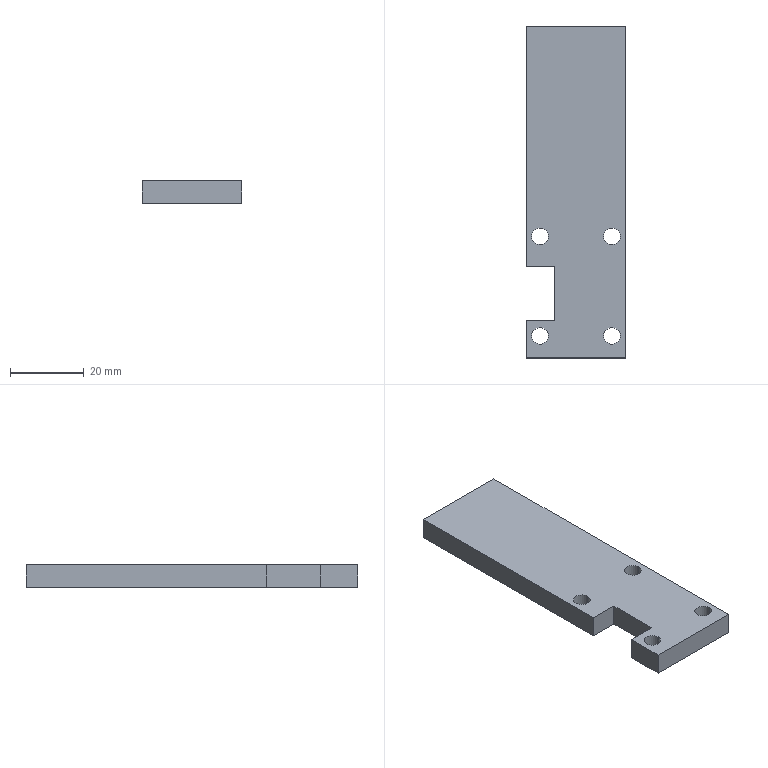Part | NX | features BREP 1 | 1 solid | 18 faces | box 27 x 90 x 6 mm | volume 13520 mm3 | plane 10 | cylinder 8 | commonest cylinder face diameters 4.5 x8
STEP:
#1=CARTESIAN_POINT('',(-758.389,33.,6.));
#2=VERTEX_POINT('',#1);
#3=CARTESIAN_POINT('',(-762.889,33.,6.));
#4=VERTEX_POINT('',#3);
#5=CARTESIAN_POINT('',(-760.639,33.,6.));
#6=DIRECTION('',(0.,0.,-1.));
#7=DIRECTION('',(-1.,0.,0.));
#8=AXIS2_PLACEMENT_3D('',#5,#6,#7);
#9=CIRCLE('',#8,2.25);
#10=EDGE_CURVE('',#2,#4,#9,.T.);
#11=ORIENTED_EDGE('',*,*,#10,.F.);
#12=CARTESIAN_POINT('',(-758.389,33.,0.));
#13=VERTEX_POINT('',#12);
#14=CARTESIAN_POINT('',(-758.389,33.,6.));
#15=DIRECTION('',(0.,0.,-1.));
#16=VECTOR('',#15,1000.);
#17=LINE('',#14,#16);
#18=EDGE_CURVE('',#2,#13,#17,.T.);
#19=ORIENTED_EDGE('',*,*,#18,.T.);
#20=CARTESIAN_POINT('',(-762.889,33.,0.));
#21=VERTEX_POINT('',#20);
#22=CARTESIAN_POINT('',(-760.639,33.,0.));
#23=DIRECTION('',(0.,0.,-1.));
#24=DIRECTION('',(-1.,0.,0.));
#25=AXIS2_PLACEMENT_3D('',#22,#23,#24);
#26=CIRCLE('',#25,2.25);
#27=EDGE_CURVE('',#13,#21,#26,.T.);
#28=ORIENTED_EDGE('',*,*,#27,.T.);
#29=CARTESIAN_POINT('',(-762.889,33.,6.));
#30=DIRECTION('',(0.,0.,-1.));
#31=VECTOR('',#30,1000.);
#32=LINE('',#29,#31);
#33=EDGE_CURVE('',#4,#21,#32,.T.);
#34=ORIENTED_EDGE('',*,*,#33,.F.);
#35=EDGE_LOOP('',(#11,#19,#28,#34));
#36=FACE_BOUND('',#35,.T.);
#37=CARTESIAN_POINT('',(-760.639,33.,6.));
#38=DIRECTION('',(0.,0.,-1.));
#39=DIRECTION('',(-1.,0.,0.));
#40=AXIS2_PLACEMENT_3D('',#37,#38,#39);
#41=CYLINDRICAL_SURFACE('',#40,2.25);
#42=ADVANCED_FACE('',(#36),#41,.F.);
#43=CARTESIAN_POINT('',(-758.389,6.,6.));
#44=VERTEX_POINT('',#43);
#45=CARTESIAN_POINT('',(-762.889,6.,6.));
#46=VERTEX_POINT('',#45);
#47=CARTESIAN_POINT('',(-760.639,6.,6.));
#48=DIRECTION('',(0.,0.,-1.));
#49=DIRECTION('',(-1.,0.,0.));
#50=AXIS2_PLACEMENT_3D('',#47,#48,#49);
#51=CIRCLE('',#50,2.25);
#52=EDGE_CURVE('',#44,#46,#51,.T.);
#53=ORIENTED_EDGE('',*,*,#52,.F.);
#54=CARTESIAN_POINT('',(-758.389,6.,0.));
#55=VERTEX_POINT('',#54);
#56=CARTESIAN_POINT('',(-758.389,6.,6.));
#57=DIRECTION('',(0.,0.,-1.));
#58=VECTOR('',#57,1000.);
#59=LINE('',#56,#58);
#60=EDGE_CURVE('',#44,#55,#59,.T.);
#61=ORIENTED_EDGE('',*,*,#60,.T.);
#62=CARTESIAN_POINT('',(-762.889,6.,0.));
#63=VERTEX_POINT('',#62);
#64=CARTESIAN_POINT('',(-760.639,6.,0.));
#65=DIRECTION('',(0.,0.,-1.));
#66=DIRECTION('',(-1.,0.,0.));
#67=AXIS2_PLACEMENT_3D('',#64,#65,#66);
#68=CIRCLE('',#67,2.25);
#69=EDGE_CURVE('',#55,#63,#68,.T.);
#70=ORIENTED_EDGE('',*,*,#69,.T.);
#71=CARTESIAN_POINT('',(-762.889,6.,6.));
#72=DIRECTION('',(0.,0.,-1.));
#73=VECTOR('',#72,1000.);
#74=LINE('',#71,#73);
#75=EDGE_CURVE('',#46,#63,#74,.T.);
#76=ORIENTED_EDGE('',*,*,#75,.F.);
#77=EDGE_LOOP('',(#53,#61,#70,#76));
#78=FACE_BOUND('',#77,.T.);
#79=CARTESIAN_POINT('',(-760.639,6.,6.));
#80=DIRECTION('',(0.,0.,-1.));
#81=DIRECTION('',(-1.,0.,0.));
#82=AXIS2_PLACEMENT_3D('',#79,#80,#81);
#83=CYLINDRICAL_SURFACE('',#82,2.25);
#84=ADVANCED_FACE('',(#78),#83,.F.);
#85=CARTESIAN_POINT('',(-777.889,6.,6.));
#86=VERTEX_POINT('',#85);
#87=CARTESIAN_POINT('',(-782.389,6.,6.));
#88=VERTEX_POINT('',#87);
#89=CARTESIAN_POINT('',(-780.139,6.,6.));
#90=DIRECTION('',(0.,0.,-1.));
#91=DIRECTION('',(-1.,0.,0.));
#92=AXIS2_PLACEMENT_3D('',#89,#90,#91);
#93=CIRCLE('',#92,2.25);
#94=EDGE_CURVE('',#86,#88,#93,.T.);
#95=ORIENTED_EDGE('',*,*,#94,.F.);
#96=CARTESIAN_POINT('',(-777.889,6.,0.));
#97=VERTEX_POINT('',#96);
#98=CARTESIAN_POINT('',(-777.889,6.,6.));
#99=DIRECTION('',(0.,0.,-1.));
#100=VECTOR('',#99,1000.);
#101=LINE('',#98,#100);
#102=EDGE_CURVE('',#86,#97,#101,.T.);
#103=ORIENTED_EDGE('',*,*,#102,.T.);
#104=CARTESIAN_POINT('',(-782.389,6.,0.));
#105=VERTEX_POINT('',#104);
#106=CARTESIAN_POINT('',(-780.139,6.,0.));
#107=DIRECTION('',(0.,0.,-1.));
#108=DIRECTION('',(-1.,0.,0.));
#109=AXIS2_PLACEMENT_3D('',#106,#107,#108);
#110=CIRCLE('',#109,2.25);
#111=EDGE_CURVE('',#97,#105,#110,.T.);
#112=ORIENTED_EDGE('',*,*,#111,.T.);
#113=CARTESIAN_POINT('',(-782.389,6.,6.));
#114=DIRECTION('',(0.,0.,-1.));
#115=VECTOR('',#114,1000.);
#116=LINE('',#113,#115);
#117=EDGE_CURVE('',#88,#105,#116,.T.);
#118=ORIENTED_EDGE('',*,*,#117,.F.);
#119=EDGE_LOOP('',(#95,#103,#112,#118));
#120=FACE_BOUND('',#119,.T.);
#121=CARTESIAN_POINT('',(-780.139,6.,6.));
#122=DIRECTION('',(0.,0.,-1.));
#123=DIRECTION('',(-1.,0.,0.));
#124=AXIS2_PLACEMENT_3D('',#121,#122,#123);
#125=CYLINDRICAL_SURFACE('',#124,2.25);
#126=ADVANCED_FACE('',(#120),#125,.F.);
#127=CARTESIAN_POINT('',(-777.889,33.,6.));
#128=VERTEX_POINT('',#127);
#129=CARTESIAN_POINT('',(-782.389,33.,6.));
#130=VERTEX_POINT('',#129);
#131=CARTESIAN_POINT('',(-780.139,33.,6.));
#132=DIRECTION('',(0.,0.,-1.));
#133=DIRECTION('',(-1.,0.,0.));
#134=AXIS2_PLACEMENT_3D('',#131,#132,#133);
#135=CIRCLE('',#134,2.25);
#136=EDGE_CURVE('',#128,#130,#135,.T.);
#137=ORIENTED_EDGE('',*,*,#136,.F.);
#138=CARTESIAN_POINT('',(-777.889,33.,0.));
#139=VERTEX_POINT('',#138);
#140=CARTESIAN_POINT('',(-777.889,33.,6.));
#141=DIRECTION('',(0.,0.,-1.));
#142=VECTOR('',#141,1000.);
#143=LINE('',#140,#142);
#144=EDGE_CURVE('',#128,#139,#143,.T.);
#145=ORIENTED_EDGE('',*,*,#144,.T.);
#146=CARTESIAN_POINT('',(-782.389,33.,0.));
#147=VERTEX_POINT('',#146);
#148=CARTESIAN_POINT('',(-780.139,33.,0.));
#149=DIRECTION('',(0.,0.,-1.));
#150=DIRECTION('',(-1.,0.,0.));
#151=AXIS2_PLACEMENT_3D('',#148,#149,#150);
#152=CIRCLE('',#151,2.25);
#153=EDGE_CURVE('',#139,#147,#152,.T.);
#154=ORIENTED_EDGE('',*,*,#153,.T.);
#155=CARTESIAN_POINT('',(-782.389,33.,6.));
#156=DIRECTION('',(0.,0.,-1.));
#157=VECTOR('',#156,1000.);
#158=LINE('',#155,#157);
#159=EDGE_CURVE('',#130,#147,#158,.T.);
#160=ORIENTED_EDGE('',*,*,#159,.F.);
#161=EDGE_LOOP('',(#137,#145,#154,#160));
#162=FACE_BOUND('',#161,.T.);
#163=CARTESIAN_POINT('',(-780.139,33.,6.));
#164=DIRECTION('',(0.,0.,-1.));
#165=DIRECTION('',(-1.,0.,0.));
#166=AXIS2_PLACEMENT_3D('',#163,#164,#165);
#167=CYLINDRICAL_SURFACE('',#166,2.25);
#168=ADVANCED_FACE('',(#162),#167,.F.);
#169=CARTESIAN_POINT('',(-783.889,10.25,6.));
#170=VERTEX_POINT('',#169);
#171=CARTESIAN_POINT('',(-783.889,0.,6.));
#172=VERTEX_POINT('',#171);
#173=CARTESIAN_POINT('',(-783.889,90.,6.));
#174=DIRECTION('',(0.,-1.,0.));
#175=VECTOR('',#174,1000.);
#176=LINE('',#173,#175);
#177=EDGE_CURVE('',#170,#172,#176,.T.);
#178=ORIENTED_EDGE('',*,*,#177,.F.);
#179=CARTESIAN_POINT('',(-783.889,10.25,0.));
#180=VERTEX_POINT('',#179);
#181=CARTESIAN_POINT('',(-783.889,10.25,0.));
#182=DIRECTION('',(0.,0.,1.));
#183=VECTOR('',#182,1000.);
#184=LINE('',#181,#183);
#185=EDGE_CURVE('',#180,#170,#184,.T.);
#186=ORIENTED_EDGE('',*,*,#185,.F.);
#187=CARTESIAN_POINT('',(-783.889,0.,0.));
#188=VERTEX_POINT('',#187);
#189=CARTESIAN_POINT('',(-783.889,90.,0.));
#190=DIRECTION('',(0.,-1.,0.));
#191=VECTOR('',#190,1000.);
#192=LINE('',#189,#191);
#193=EDGE_CURVE('',#180,#188,#192,.T.);
#194=ORIENTED_EDGE('',*,*,#193,.T.);
#195=CARTESIAN_POINT('',(-783.889,0.,6.));
#196=DIRECTION('',(0.,0.,-1.));
#197=VECTOR('',#196,1000.);
#198=LINE('',#195,#197);
#199=EDGE_CURVE('',#172,#188,#198,.T.);
#200=ORIENTED_EDGE('',*,*,#199,.F.);
#201=EDGE_LOOP('',(#178,#186,#194,#200));
#202=FACE_BOUND('',#201,.T.);
#203=CARTESIAN_POINT('',(-783.889,90.,6.));
#204=DIRECTION('',(1.,0.,0.));
#205=DIRECTION('',(0.,1.,0.));
#206=AXIS2_PLACEMENT_3D('',#203,#204,#205);
#207=PLANE('',#206);
#208=ADVANCED_FACE('',(#202),#207,.F.);
#209=CARTESIAN_POINT('',(-756.889,0.,0.));
#210=VERTEX_POINT('',#209);
#211=CARTESIAN_POINT('',(-756.889,90.,0.));
#212=VERTEX_POINT('',#211);
#213=CARTESIAN_POINT('',(-756.889,90.,0.));
#214=DIRECTION('',(0.,1.,0.));
#215=VECTOR('',#214,1000.);
#216=LINE('',#213,#215);
#217=EDGE_CURVE('',#210,#212,#216,.T.);
#218=ORIENTED_EDGE('',*,*,#217,.T.);
#219=CARTESIAN_POINT('',(-756.889,90.,6.));
#220=VERTEX_POINT('',#219);
#221=CARTESIAN_POINT('',(-756.889,90.,6.));
#222=DIRECTION('',(0.,0.,-1.));
#223=VECTOR('',#222,1000.);
#224=LINE('',#221,#223);
#225=EDGE_CURVE('',#220,#212,#224,.T.);
#226=ORIENTED_EDGE('',*,*,#225,.F.);
#227=CARTESIAN_POINT('',(-756.889,0.,6.));
#228=VERTEX_POINT('',#227);
#229=CARTESIAN_POINT('',(-756.889,90.,6.));
#230=DIRECTION('',(0.,1.,0.));
#231=VECTOR('',#230,1000.);
#232=LINE('',#229,#231);
#233=EDGE_CURVE('',#228,#220,#232,.T.);
#234=ORIENTED_EDGE('',*,*,#233,.F.);
#235=CARTESIAN_POINT('',(-756.889,0.,6.));
#236=DIRECTION('',(0.,0.,-1.));
#237=VECTOR('',#236,1000.);
#238=LINE('',#235,#237);
#239=EDGE_CURVE('',#228,#210,#238,.T.);
#240=ORIENTED_EDGE('',*,*,#239,.T.);
#241=EDGE_LOOP('',(#218,#226,#234,#240));
#242=FACE_BOUND('',#241,.T.);
#243=CARTESIAN_POINT('',(-756.889,90.,6.));
#244=DIRECTION('',(-1.,0.,0.));
#245=DIRECTION('',(0.,0.,1.));
#246=AXIS2_PLACEMENT_3D('',#243,#244,#245);
#247=PLANE('',#246);
#248=ADVANCED_FACE('',(#242),#247,.F.);
#249=CARTESIAN_POINT('',(-783.889,90.,0.));
#250=VERTEX_POINT('',#249);
#251=CARTESIAN_POINT('',(-756.889,90.,0.));
#252=DIRECTION('',(-1.,0.,0.));
#253=VECTOR('',#252,1000.);
#254=LINE('',#251,#253);
#255=EDGE_CURVE('',#212,#250,#254,.T.);
#256=ORIENTED_EDGE('',*,*,#255,.T.);
#257=CARTESIAN_POINT('',(-783.889,90.,6.));
#258=VERTEX_POINT('',#257);
#259=CARTESIAN_POINT('',(-783.889,90.,6.));
#260=DIRECTION('',(0.,0.,-1.));
#261=VECTOR('',#260,1000.);
#262=LINE('',#259,#261);
#263=EDGE_CURVE('',#258,#250,#262,.T.);
#264=ORIENTED_EDGE('',*,*,#263,.F.);
#265=CARTESIAN_POINT('',(-756.889,90.,6.));
#266=DIRECTION('',(-1.,0.,0.));
#267=VECTOR('',#266,1000.);
#268=LINE('',#265,#267);
#269=EDGE_CURVE('',#220,#258,#268,.T.);
#270=ORIENTED_EDGE('',*,*,#269,.F.);
#271=ORIENTED_EDGE('',*,*,#225,.T.);
#272=EDGE_LOOP('',(#256,#264,#270,#271));
#273=FACE_BOUND('',#272,.T.);
#274=CARTESIAN_POINT('',(-756.889,90.,6.));
#275=DIRECTION('',(0.,-1.,0.));
#276=DIRECTION('',(0.,0.,-1.));
#277=AXIS2_PLACEMENT_3D('',#274,#275,#276);
#278=PLANE('',#277);
#279=ADVANCED_FACE('',(#273),#278,.F.);
#280=CARTESIAN_POINT('',(-783.889,24.75,0.));
#281=VERTEX_POINT('',#280);
#282=CARTESIAN_POINT('',(-783.889,90.,0.));
#283=DIRECTION('',(0.,-1.,0.));
#284=VECTOR('',#283,1000.);
#285=LINE('',#282,#284);
#286=EDGE_CURVE('',#250,#281,#285,.T.);
#287=ORIENTED_EDGE('',*,*,#286,.T.);
#288=CARTESIAN_POINT('',(-783.889,24.75,6.));
#289=VERTEX_POINT('',#288);
#290=CARTESIAN_POINT('',(-783.889,24.75,0.));
#291=DIRECTION('',(0.,0.,1.));
#292=VECTOR('',#291,1000.);
#293=LINE('',#290,#292);
#294=EDGE_CURVE('',#281,#289,#293,.T.);
#295=ORIENTED_EDGE('',*,*,#294,.T.);
#296=CARTESIAN_POINT('',(-783.889,90.,6.));
#297=DIRECTION('',(0.,-1.,0.));
#298=VECTOR('',#297,1000.);
#299=LINE('',#296,#298);
#300=EDGE_CURVE('',#258,#289,#299,.T.);
#301=ORIENTED_EDGE('',*,*,#300,.F.);
#302=ORIENTED_EDGE('',*,*,#263,.T.);
#303=EDGE_LOOP('',(#287,#295,#301,#302));
#304=FACE_BOUND('',#303,.T.);
#305=CARTESIAN_POINT('',(-783.889,90.,6.));
#306=DIRECTION('',(1.,0.,0.));
#307=DIRECTION('',(0.,1.,0.));
#308=AXIS2_PLACEMENT_3D('',#305,#306,#307);
#309=PLANE('',#308);
#310=ADVANCED_FACE('',(#304),#309,.F.);
#311=CARTESIAN_POINT('',(-756.889,0.,0.));
#312=DIRECTION('',(1.,0.,0.));
#313=VECTOR('',#312,1000.);
#314=LINE('',#311,#313);
#315=EDGE_CURVE('',#188,#210,#314,.T.);
#316=ORIENTED_EDGE('',*,*,#315,.T.);
#317=ORIENTED_EDGE('',*,*,#239,.F.);
#318=CARTESIAN_POINT('',(-756.889,0.,6.));
#319=DIRECTION('',(1.,0.,0.));
#320=VECTOR('',#319,1000.);
#321=LINE('',#318,#320);
#322=EDGE_CURVE('',#172,#228,#321,.T.);
#323=ORIENTED_EDGE('',*,*,#322,.F.);
#324=ORIENTED_EDGE('',*,*,#199,.T.);
#325=EDGE_LOOP('',(#316,#317,#323,#324));
#326=FACE_BOUND('',#325,.T.);
#327=CARTESIAN_POINT('',(-756.889,0.,6.));
#328=DIRECTION('',(0.,1.,0.));
#329=DIRECTION('',(1.,0.,0.));
#330=AXIS2_PLACEMENT_3D('',#327,#328,#329);
#331=PLANE('',#330);
#332=ADVANCED_FACE('',(#326),#331,.F.);
#333=CARTESIAN_POINT('',(-776.089,10.25,6.));
#334=VERTEX_POINT('',#333);
#335=CARTESIAN_POINT('',(-776.089,24.75,6.));
#336=VERTEX_POINT('',#335);
#337=CARTESIAN_POINT('',(-776.089,10.25,6.));
#338=DIRECTION('',(0.,1.,0.));
#339=VECTOR('',#338,1000.);
#340=LINE('',#337,#339);
#341=EDGE_CURVE('',#334,#336,#340,.T.);
#342=ORIENTED_EDGE('',*,*,#341,.F.);
#343=CARTESIAN_POINT('',(-776.089,10.25,6.));
#344=DIRECTION('',(1.,0.,0.));
#345=VECTOR('',#344,1000.);
#346=LINE('',#343,#345);
#347=EDGE_CURVE('',#170,#334,#346,.T.);
#348=ORIENTED_EDGE('',*,*,#347,.F.);
#349=ORIENTED_EDGE('',*,*,#177,.T.);
#350=ORIENTED_EDGE('',*,*,#322,.T.);
#351=ORIENTED_EDGE('',*,*,#233,.T.);
#352=ORIENTED_EDGE('',*,*,#269,.T.);
#353=ORIENTED_EDGE('',*,*,#300,.T.);
#354=CARTESIAN_POINT('',(-776.089,24.75,6.));
#355=DIRECTION('',(-1.,0.,0.));
#356=VECTOR('',#355,1000.);
#357=LINE('',#354,#356);
#358=EDGE_CURVE('',#336,#289,#357,.T.);
#359=ORIENTED_EDGE('',*,*,#358,.F.);
#360=EDGE_LOOP('',(#342,#348,#349,#350,#351,#352,#353,#359));
#361=FACE_BOUND('',#360,.T.);
#362=CARTESIAN_POINT('',(-760.639,33.,6.));
#363=DIRECTION('',(0.,0.,-1.));
#364=DIRECTION('',(-1.,0.,0.));
#365=AXIS2_PLACEMENT_3D('',#362,#363,#364);
#366=CIRCLE('',#365,2.25);
#367=EDGE_CURVE('',#4,#2,#366,.T.);
#368=ORIENTED_EDGE('',*,*,#367,.T.);
#369=ORIENTED_EDGE('',*,*,#10,.T.);
#370=EDGE_LOOP('',(#368,#369));
#371=FACE_BOUND('',#370,.T.);
#372=CARTESIAN_POINT('',(-760.639,6.,6.));
#373=DIRECTION('',(0.,0.,-1.));
#374=DIRECTION('',(-1.,0.,0.));
#375=AXIS2_PLACEMENT_3D('',#372,#373,#374);
#376=CIRCLE('',#375,2.25);
#377=EDGE_CURVE('',#46,#44,#376,.T.);
#378=ORIENTED_EDGE('',*,*,#377,.T.);
#379=ORIENTED_EDGE('',*,*,#52,.T.);
#380=EDGE_LOOP('',(#378,#379));
#381=FACE_BOUND('',#380,.T.);
#382=CARTESIAN_POINT('',(-780.139,6.,6.));
#383=DIRECTION('',(0.,0.,-1.));
#384=DIRECTION('',(-1.,0.,0.));
#385=AXIS2_PLACEMENT_3D('',#382,#383,#384);
#386=CIRCLE('',#385,2.25);
#387=EDGE_CURVE('',#88,#86,#386,.T.);
#388=ORIENTED_EDGE('',*,*,#387,.T.);
#389=ORIENTED_EDGE('',*,*,#94,.T.);
#390=EDGE_LOOP('',(#388,#389));
#391=FACE_BOUND('',#390,.T.);
#392=CARTESIAN_POINT('',(-780.139,33.,6.));
#393=DIRECTION('',(0.,0.,-1.));
#394=DIRECTION('',(-1.,0.,0.));
#395=AXIS2_PLACEMENT_3D('',#392,#393,#394);
#396=CIRCLE('',#395,2.25);
#397=EDGE_CURVE('',#130,#128,#396,.T.);
#398=ORIENTED_EDGE('',*,*,#397,.T.);
#399=ORIENTED_EDGE('',*,*,#136,.T.);
#400=EDGE_LOOP('',(#398,#399));
#401=FACE_BOUND('',#400,.T.);
#402=CARTESIAN_POINT('',(-756.889,0.,6.));
#403=DIRECTION('',(0.,0.,-1.));
#404=DIRECTION('',(0.,-1.,0.));
#405=AXIS2_PLACEMENT_3D('',#402,#403,#404);
#406=PLANE('',#405);
#407=ADVANCED_FACE('',(#361,#371,#381,#391,#401),#406,.F.);
#408=CARTESIAN_POINT('',(-776.089,10.25,0.));
#409=VERTEX_POINT('',#408);
#410=CARTESIAN_POINT('',(-776.089,10.25,0.));
#411=DIRECTION('',(1.,0.,0.));
#412=VECTOR('',#411,1000.);
#413=LINE('',#410,#412);
#414=EDGE_CURVE('',#180,#409,#413,.T.);
#415=ORIENTED_EDGE('',*,*,#414,.T.);
#416=CARTESIAN_POINT('',(-776.089,24.75,0.));
#417=VERTEX_POINT('',#416);
#418=CARTESIAN_POINT('',(-776.089,10.25,0.));
#419=DIRECTION('',(0.,1.,0.));
#420=VECTOR('',#419,1000.);
#421=LINE('',#418,#420);
#422=EDGE_CURVE('',#409,#417,#421,.T.);
#423=ORIENTED_EDGE('',*,*,#422,.T.);
#424=CARTESIAN_POINT('',(-776.089,24.75,0.));
#425=DIRECTION('',(-1.,0.,0.));
#426=VECTOR('',#425,1000.);
#427=LINE('',#424,#426);
#428=EDGE_CURVE('',#417,#281,#427,.T.);
#429=ORIENTED_EDGE('',*,*,#428,.T.);
#430=ORIENTED_EDGE('',*,*,#286,.F.);
#431=ORIENTED_EDGE('',*,*,#255,.F.);
#432=ORIENTED_EDGE('',*,*,#217,.F.);
#433=ORIENTED_EDGE('',*,*,#315,.F.);
#434=ORIENTED_EDGE('',*,*,#193,.F.);
#435=EDGE_LOOP('',(#415,#423,#429,#430,#431,#432,#433,#434));
#436=FACE_BOUND('',#435,.T.);
#437=CARTESIAN_POINT('',(-760.639,33.,0.));
#438=DIRECTION('',(0.,0.,-1.));
#439=DIRECTION('',(-1.,0.,0.));
#440=AXIS2_PLACEMENT_3D('',#437,#438,#439);
#441=CIRCLE('',#440,2.25);
#442=EDGE_CURVE('',#21,#13,#441,.T.);
#443=ORIENTED_EDGE('',*,*,#442,.F.);
#444=ORIENTED_EDGE('',*,*,#27,.F.);
#445=EDGE_LOOP('',(#443,#444));
#446=FACE_BOUND('',#445,.T.);
#447=CARTESIAN_POINT('',(-760.639,6.,0.));
#448=DIRECTION('',(0.,0.,-1.));
#449=DIRECTION('',(-1.,0.,0.));
#450=AXIS2_PLACEMENT_3D('',#447,#448,#449);
#451=CIRCLE('',#450,2.25);
#452=EDGE_CURVE('',#63,#55,#451,.T.);
#453=ORIENTED_EDGE('',*,*,#452,.F.);
#454=ORIENTED_EDGE('',*,*,#69,.F.);
#455=EDGE_LOOP('',(#453,#454));
#456=FACE_BOUND('',#455,.T.);
#457=CARTESIAN_POINT('',(-780.139,6.,0.));
#458=DIRECTION('',(0.,0.,-1.));
#459=DIRECTION('',(-1.,0.,0.));
#460=AXIS2_PLACEMENT_3D('',#457,#458,#459);
#461=CIRCLE('',#460,2.25);
#462=EDGE_CURVE('',#105,#97,#461,.T.);
#463=ORIENTED_EDGE('',*,*,#462,.F.);
#464=ORIENTED_EDGE('',*,*,#111,.F.);
#465=EDGE_LOOP('',(#463,#464));
#466=FACE_BOUND('',#465,.T.);
#467=CARTESIAN_POINT('',(-780.139,33.,0.));
#468=DIRECTION('',(0.,0.,-1.));
#469=DIRECTION('',(-1.,0.,0.));
#470=AXIS2_PLACEMENT_3D('',#467,#468,#469);
#471=CIRCLE('',#470,2.25);
#472=EDGE_CURVE('',#147,#139,#471,.T.);
#473=ORIENTED_EDGE('',*,*,#472,.F.);
#474=ORIENTED_EDGE('',*,*,#153,.F.);
#475=EDGE_LOOP('',(#473,#474));
#476=FACE_BOUND('',#475,.T.);
#477=CARTESIAN_POINT('',(-756.889,0.,0.));
#478=DIRECTION('',(0.,0.,-1.));
#479=DIRECTION('',(0.,-1.,0.));
#480=AXIS2_PLACEMENT_3D('',#477,#478,#479);
#481=PLANE('',#480);
#482=ADVANCED_FACE('',(#436,#446,#456,#466,#476),#481,.T.);
#483=ORIENTED_EDGE('',*,*,#144,.F.);
#484=ORIENTED_EDGE('',*,*,#397,.F.);
#485=ORIENTED_EDGE('',*,*,#159,.T.);
#486=ORIENTED_EDGE('',*,*,#472,.T.);
#487=EDGE_LOOP('',(#483,#484,#485,#486));
#488=FACE_BOUND('',#487,.T.);
#489=CARTESIAN_POINT('',(-780.139,33.,6.));
#490=DIRECTION('',(0.,0.,-1.));
#491=DIRECTION('',(-1.,0.,0.));
#492=AXIS2_PLACEMENT_3D('',#489,#490,#491);
#493=CYLINDRICAL_SURFACE('',#492,2.25);
#494=ADVANCED_FACE('',(#488),#493,.F.);
#495=ORIENTED_EDGE('',*,*,#102,.F.);
#496=ORIENTED_EDGE('',*,*,#387,.F.);
#497=ORIENTED_EDGE('',*,*,#117,.T.);
#498=ORIENTED_EDGE('',*,*,#462,.T.);
#499=EDGE_LOOP('',(#495,#496,#497,#498));
#500=FACE_BOUND('',#499,.T.);
#501=CARTESIAN_POINT('',(-780.139,6.,6.));
#502=DIRECTION('',(0.,0.,-1.));
#503=DIRECTION('',(-1.,0.,0.));
#504=AXIS2_PLACEMENT_3D('',#501,#502,#503);
#505=CYLINDRICAL_SURFACE('',#504,2.25);
#506=ADVANCED_FACE('',(#500),#505,.F.);
#507=ORIENTED_EDGE('',*,*,#60,.F.);
#508=ORIENTED_EDGE('',*,*,#377,.F.);
#509=ORIENTED_EDGE('',*,*,#75,.T.);
#510=ORIENTED_EDGE('',*,*,#452,.T.);
#511=EDGE_LOOP('',(#507,#508,#509,#510));
#512=FACE_BOUND('',#511,.T.);
#513=CARTESIAN_POINT('',(-760.639,6.,6.));
#514=DIRECTION('',(0.,0.,-1.));
#515=DIRECTION('',(-1.,0.,0.));
#516=AXIS2_PLACEMENT_3D('',#513,#514,#515);
#517=CYLINDRICAL_SURFACE('',#516,2.25);
#518=ADVANCED_FACE('',(#512),#517,.F.);
#519=ORIENTED_EDGE('',*,*,#18,.F.);
#520=ORIENTED_EDGE('',*,*,#367,.F.);
#521=ORIENTED_EDGE('',*,*,#33,.T.);
#522=ORIENTED_EDGE('',*,*,#442,.T.);
#523=EDGE_LOOP('',(#519,#520,#521,#522));
#524=FACE_BOUND('',#523,.T.);
#525=CARTESIAN_POINT('',(-760.639,33.,6.));
#526=DIRECTION('',(0.,0.,-1.));
#527=DIRECTION('',(-1.,0.,0.));
#528=AXIS2_PLACEMENT_3D('',#525,#526,#527);
#529=CYLINDRICAL_SURFACE('',#528,2.25);
#530=ADVANCED_FACE('',(#524),#529,.F.);
#531=ORIENTED_EDGE('',*,*,#341,.T.);
#532=CARTESIAN_POINT('',(-776.089,24.75,0.));
#533=DIRECTION('',(0.,0.,1.));
#534=VECTOR('',#533,1000.);
#535=LINE('',#532,#534);
#536=EDGE_CURVE('',#417,#336,#535,.T.);
#537=ORIENTED_EDGE('',*,*,#536,.F.);
#538=ORIENTED_EDGE('',*,*,#422,.F.);
#539=CARTESIAN_POINT('',(-776.089,10.25,0.));
#540=DIRECTION('',(0.,0.,1.));
#541=VECTOR('',#540,1000.);
#542=LINE('',#539,#541);
#543=EDGE_CURVE('',#409,#334,#542,.T.);
#544=ORIENTED_EDGE('',*,*,#543,.T.);
#545=EDGE_LOOP('',(#531,#537,#538,#544));
#546=FACE_BOUND('',#545,.T.);
#547=CARTESIAN_POINT('',(-776.089,10.25,0.));
#548=DIRECTION('',(1.,0.,0.));
#549=DIRECTION('',(0.,1.,0.));
#550=AXIS2_PLACEMENT_3D('',#547,#548,#549);
#551=PLANE('',#550);
#552=ADVANCED_FACE('',(#546),#551,.F.);
#553=ORIENTED_EDGE('',*,*,#347,.T.);
#554=ORIENTED_EDGE('',*,*,#543,.F.);
#555=ORIENTED_EDGE('',*,*,#414,.F.);
#556=ORIENTED_EDGE('',*,*,#185,.T.);
#557=EDGE_LOOP('',(#553,#554,#555,#556));
#558=FACE_BOUND('',#557,.T.);
#559=CARTESIAN_POINT('',(-776.089,10.25,0.));
#560=DIRECTION('',(0.,-1.,0.));
#561=DIRECTION('',(0.,0.,-1.));
#562=AXIS2_PLACEMENT_3D('',#559,#560,#561);
#563=PLANE('',#562);
#564=ADVANCED_FACE('',(#558),#563,.F.);
#565=ORIENTED_EDGE('',*,*,#358,.T.);
#566=ORIENTED_EDGE('',*,*,#294,.F.);
#567=ORIENTED_EDGE('',*,*,#428,.F.);
#568=ORIENTED_EDGE('',*,*,#536,.T.);
#569=EDGE_LOOP('',(#565,#566,#567,#568));
#570=FACE_BOUND('',#569,.T.);
#571=CARTESIAN_POINT('',(-776.089,24.75,0.));
#572=DIRECTION('',(0.,1.,0.));
#573=DIRECTION('',(1.,0.,0.));
#574=AXIS2_PLACEMENT_3D('',#571,#572,#573);
#575=PLANE('',#574);
#576=ADVANCED_FACE('',(#570),#575,.F.);
#577=CLOSED_SHELL('',(#42,#84,#126,#168,#208,#248,#279,#310,#332,#407,#482,#494,#506,#518,#530,#552,#564,#576));
#578=MANIFOLD_SOLID_BREP('',#577);
#579=(LENGTH_UNIT()NAMED_UNIT(*)SI_UNIT(.MILLI.,.METRE.));
#580=UNCERTAINTY_MEASURE_WITH_UNIT(LENGTH_MEASURE(0.00001),#579,'','');
#581=(NAMED_UNIT(*)PLANE_ANGLE_UNIT()SI_UNIT($,.RADIAN.));
#582=(NAMED_UNIT(*)SI_UNIT($,.STERADIAN.)SOLID_ANGLE_UNIT());
#583=(GEOMETRIC_REPRESENTATION_CONTEXT(3)GLOBAL_UNCERTAINTY_ASSIGNED_CONTEXT((#580))GLOBAL_UNIT_ASSIGNED_CONTEXT((#579,#581,#582))REPRESENTATION_CONTEXT('',''));
#584=ADVANCED_BREP_SHAPE_REPRESENTATION('',(#578),#583);